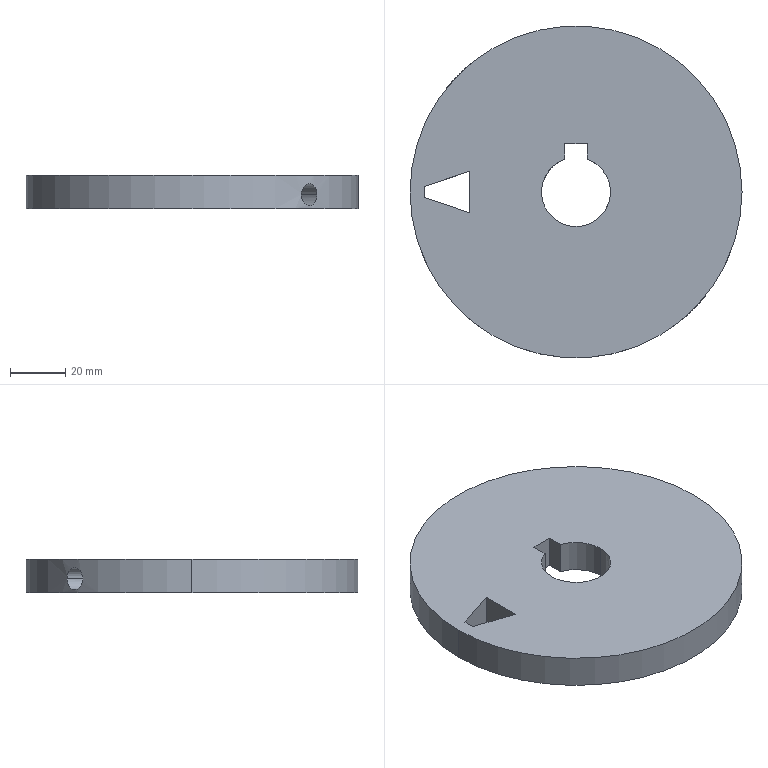Part | 1 solid | 24 faces | box 120 x 120 x 12 mm | volume 123752 mm3 | cylinder 13 | plane 11 | commonest cylinder face diameters 5 x4 8 x4 25 x3 120 x2
STEP:
#1=CARTESIAN_POINT('',(-45.16,39.504,5.));
#2=VERTEX_POINT('',#1);
#3=CARTESIAN_POINT('',(-39.504,45.16,5.));
#4=VERTEX_POINT('',#3);
#5=CARTESIAN_POINT('',(-45.16,39.504,5.));
#6=CARTESIAN_POINT('',(-45.16,39.504,4.739));
#7=CARTESIAN_POINT('',(-45.144,39.523,4.479));
#8=CARTESIAN_POINT('',(-45.076,39.6,3.964));
#9=CARTESIAN_POINT('',(-45.025,39.658,3.711));
#10=CARTESIAN_POINT('',(-44.893,39.807,3.23));
#11=CARTESIAN_POINT('',(-44.811,39.9,2.997));
#12=CARTESIAN_POINT('',(-44.616,40.118,2.559));
#13=CARTESIAN_POINT('',(-44.505,40.241,2.358));
#14=CARTESIAN_POINT('',(-44.256,40.514,1.989));
#15=CARTESIAN_POINT('',(-44.117,40.666,1.82));
#16=CARTESIAN_POINT('',(-43.821,40.985,1.529));
#17=CARTESIAN_POINT('',(-43.664,41.152,1.406));
#18=CARTESIAN_POINT('',(-43.331,41.503,1.206));
#19=CARTESIAN_POINT('',(-43.155,41.686,1.128));
#20=CARTESIAN_POINT('',(-42.798,42.053,1.026));
#21=CARTESIAN_POINT('',(-42.615,42.237,1.));
#22=CARTESIAN_POINT('',(-42.242,42.611,0.9998));
#23=CARTESIAN_POINT('',(-42.056,42.794,1.026));
#24=CARTESIAN_POINT('',(-41.69,43.151,1.127));
#25=CARTESIAN_POINT('',(-41.507,43.327,1.203));
#26=CARTESIAN_POINT('',(-41.156,43.661,1.404));
#27=CARTESIAN_POINT('',(-40.988,43.818,1.527));
#28=CARTESIAN_POINT('',(-40.669,44.114,1.816));
#29=CARTESIAN_POINT('',(-40.517,44.253,1.985));
#30=CARTESIAN_POINT('',(-40.244,44.502,2.354));
#31=CARTESIAN_POINT('',(-40.121,44.613,2.555));
#32=CARTESIAN_POINT('',(-39.902,44.809,2.992));
#33=CARTESIAN_POINT('',(-39.809,44.892,3.225));
#34=CARTESIAN_POINT('',(-39.659,45.024,3.706));
#35=CARTESIAN_POINT('',(-39.601,45.075,3.957));
#36=CARTESIAN_POINT('',(-39.523,45.143,4.474));
#37=CARTESIAN_POINT('',(-39.504,45.16,4.736));
#38=CARTESIAN_POINT('',(-39.504,45.16,5.));
#39=B_SPLINE_CURVE_WITH_KNOTS('',3,(#5,#6,#7,#8,#9,#10,#11,#12,#13,#14,#15,#16,#17,#18,#19,#20,#21,#22,#23,#24,#25,#26,#27,#28,#29,#30,#31,#32,#33,#34,#35,#36,#37,#38),.UNSPECIFIED.,.F.,.F.,(4,2,2,2,2,2,2,2,2,2,2,2,2,2,2,2,4),(0.01251,0.01329,0.01407,0.01485,0.01564,0.01642,0.0172,0.01798,0.01876,0.01954,0.02033,0.02111,0.02189,0.02267,0.02345,0.02423,0.02502),.UNSPECIFIED.);
#40=EDGE_CURVE('',#2,#4,#39,.T.);
#41=ORIENTED_EDGE('',*,*,#40,.F.);
#42=CARTESIAN_POINT('',(-24.042,18.385,5.));
#43=VERTEX_POINT('',#42);
#44=CARTESIAN_POINT('',(-58.69,53.033,5.));
#45=DIRECTION('',(0.7071,-0.7071,0.));
#46=VECTOR('',#45,1000.);
#47=LINE('',#44,#46);
#48=EDGE_CURVE('',#2,#43,#47,.T.);
#49=ORIENTED_EDGE('',*,*,#48,.T.);
#50=CARTESIAN_POINT('',(-18.385,24.042,5.));
#51=VERTEX_POINT('',#50);
#52=CARTESIAN_POINT('',(-21.213,21.213,5.));
#53=DIRECTION('',(0.7071,-0.7071,0.));
#54=DIRECTION('',(0.7071,0.7071,0.));
#55=AXIS2_PLACEMENT_3D('',#52,#53,#54);
#56=CIRCLE('',#55,4.);
#57=EDGE_CURVE('',#43,#51,#56,.T.);
#58=ORIENTED_EDGE('',*,*,#57,.T.);
#59=CARTESIAN_POINT('',(-53.033,58.69,5.));
#60=DIRECTION('',(0.7071,-0.7071,0.));
#61=VECTOR('',#60,1000.);
#62=LINE('',#59,#61);
#63=EDGE_CURVE('',#4,#51,#62,.T.);
#64=ORIENTED_EDGE('',*,*,#63,.F.);
#65=EDGE_LOOP('',(#41,#49,#58,#64));
#66=FACE_OUTER_BOUND('',#65,.T.);
#67=CARTESIAN_POINT('',(-55.861,55.861,5.));
#68=DIRECTION('',(0.7071,-0.7071,0.));
#69=DIRECTION('',(0.7071,0.7071,0.));
#70=AXIS2_PLACEMENT_3D('',#67,#68,#69);
#71=CYLINDRICAL_SURFACE('',#70,4.);
#72=ADVANCED_FACE('',(#66),#71,.F.);
#73=CARTESIAN_POINT('',(39.504,-45.16,5.));
#74=VERTEX_POINT('',#73);
#75=CARTESIAN_POINT('',(45.16,-39.504,5.));
#76=VERTEX_POINT('',#75);
#77=CARTESIAN_POINT('',(39.504,-45.16,5.));
#78=CARTESIAN_POINT('',(39.504,-45.16,4.736));
#79=CARTESIAN_POINT('',(39.523,-45.143,4.476));
#80=CARTESIAN_POINT('',(39.6,-45.076,3.964));
#81=CARTESIAN_POINT('',(39.658,-45.025,3.71));
#82=CARTESIAN_POINT('',(39.809,-44.892,3.226));
#83=CARTESIAN_POINT('',(39.901,-44.81,2.996));
#84=CARTESIAN_POINT('',(40.117,-44.616,2.561));
#85=CARTESIAN_POINT('',(40.243,-44.503,2.355));
#86=CARTESIAN_POINT('',(40.516,-44.255,1.987));
#87=CARTESIAN_POINT('',(40.665,-44.118,1.821));
#88=CARTESIAN_POINT('',(40.985,-43.821,1.529));
#89=CARTESIAN_POINT('',(41.155,-43.661,1.404));
#90=CARTESIAN_POINT('',(41.504,-43.33,1.205));
#91=CARTESIAN_POINT('',(41.686,-43.155,1.128));
#92=CARTESIAN_POINT('',(42.056,-42.794,1.025));
#93=CARTESIAN_POINT('',(42.241,-42.612,1.));
#94=CARTESIAN_POINT('',(42.61,-42.243,0.9999));
#95=CARTESIAN_POINT('',(42.796,-42.054,1.026));
#96=CARTESIAN_POINT('',(43.154,-41.687,1.128));
#97=CARTESIAN_POINT('',(43.327,-41.507,1.204));
#98=CARTESIAN_POINT('',(43.661,-41.156,1.404));
#99=CARTESIAN_POINT('',(43.821,-40.985,1.529));
#100=CARTESIAN_POINT('',(44.116,-40.667,1.819));
#101=CARTESIAN_POINT('',(44.253,-40.518,1.984));
#102=CARTESIAN_POINT('',(44.505,-40.241,2.358));
#103=CARTESIAN_POINT('',(44.616,-40.118,2.56));
#104=CARTESIAN_POINT('',(44.809,-39.902,2.993));
#105=CARTESIAN_POINT('',(44.892,-39.808,3.227));
#106=CARTESIAN_POINT('',(45.026,-39.657,3.712));
#107=CARTESIAN_POINT('',(45.076,-39.6,3.961));
#108=CARTESIAN_POINT('',(45.143,-39.523,4.474));
#109=CARTESIAN_POINT('',(45.16,-39.504,4.739));
#110=CARTESIAN_POINT('',(45.16,-39.504,5.));
#111=B_SPLINE_CURVE_WITH_KNOTS('',3,(#77,#78,#79,#80,#81,#82,#83,#84,#85,#86,#87,#88,#89,#90,#91,#92,#93,#94,#95,#96,#97,#98,#99,#100,#101,#102,#103,#104,#105,#106,#107,#108,#109,#110),.UNSPECIFIED.,.F.,.F.,(4,2,2,2,2,2,2,2,2,2,2,2,2,2,2,2,4),(0.,0.0007818,0.001564,0.002345,0.003127,0.003909,0.004691,0.005473,0.006255,0.007036,0.007818,0.0086,0.009382,0.01016,0.01095,0.01173,0.01251),.UNSPECIFIED.);
#112=EDGE_CURVE('',#74,#76,#111,.T.);
#113=ORIENTED_EDGE('',*,*,#112,.T.);
#114=CARTESIAN_POINT('',(24.042,-18.385,5.));
#115=VERTEX_POINT('',#114);
#116=CARTESIAN_POINT('',(58.69,-53.033,5.));
#117=DIRECTION('',(-0.7071,0.7071,0.));
#118=VECTOR('',#117,1000.);
#119=LINE('',#116,#118);
#120=EDGE_CURVE('',#76,#115,#119,.T.);
#121=ORIENTED_EDGE('',*,*,#120,.T.);
#122=CARTESIAN_POINT('',(18.385,-24.042,5.));
#123=VERTEX_POINT('',#122);
#124=CARTESIAN_POINT('',(21.213,-21.213,5.));
#125=DIRECTION('',(0.7071,-0.7071,0.));
#126=DIRECTION('',(0.7071,0.7071,0.));
#127=AXIS2_PLACEMENT_3D('',#124,#125,#126);
#128=CIRCLE('',#127,4.);
#129=EDGE_CURVE('',#123,#115,#128,.T.);
#130=ORIENTED_EDGE('',*,*,#129,.F.);
#131=CARTESIAN_POINT('',(53.033,-58.69,5.));
#132=DIRECTION('',(-0.7071,0.7071,0.));
#133=VECTOR('',#132,1000.);
#134=LINE('',#131,#133);
#135=EDGE_CURVE('',#74,#123,#134,.T.);
#136=ORIENTED_EDGE('',*,*,#135,.F.);
#137=EDGE_LOOP('',(#113,#121,#130,#136));
#138=FACE_OUTER_BOUND('',#137,.T.);
#139=CARTESIAN_POINT('',(55.861,-55.861,5.));
#140=DIRECTION('',(-0.7071,0.7071,0.));
#141=DIRECTION('',(-0.7071,-0.7071,0.));
#142=AXIS2_PLACEMENT_3D('',#139,#140,#141);
#143=CYLINDRICAL_SURFACE('',#142,4.);
#144=ADVANCED_FACE('',(#138),#143,.F.);
#145=CARTESIAN_POINT('',(6.892,-10.428,5.));
#146=VERTEX_POINT('',#145);
#147=CARTESIAN_POINT('',(10.428,-6.892,5.));
#148=VERTEX_POINT('',#147);
#149=CARTESIAN_POINT('',(6.892,-10.428,5.));
#150=CARTESIAN_POINT('',(6.892,-10.428,4.834));
#151=CARTESIAN_POINT('',(6.906,-10.419,4.672));
#152=CARTESIAN_POINT('',(6.961,-10.383,4.351));
#153=CARTESIAN_POINT('',(7.001,-10.355,4.192));
#154=CARTESIAN_POINT('',(7.107,-10.283,3.89));
#155=CARTESIAN_POINT('',(7.171,-10.239,3.746));
#156=CARTESIAN_POINT('',(7.321,-10.132,3.475));
#157=CARTESIAN_POINT('',(7.407,-10.069,3.347));
#158=CARTESIAN_POINT('',(7.686,-9.86,3.002));
#159=CARTESIAN_POINT('',(7.906,-9.687,2.816));
#160=CARTESIAN_POINT('',(8.25,-9.392,2.629));
#161=CARTESIAN_POINT('',(8.368,-9.287,2.58));
#162=CARTESIAN_POINT('',(8.605,-9.068,2.516));
#163=CARTESIAN_POINT('',(8.723,-8.955,2.5));
#164=CARTESIAN_POINT('',(8.954,-8.724,2.5));
#165=CARTESIAN_POINT('',(9.069,-8.604,2.516));
#166=CARTESIAN_POINT('',(9.287,-8.368,2.58));
#167=CARTESIAN_POINT('',(9.391,-8.251,2.628));
#168=CARTESIAN_POINT('',(9.589,-8.02,2.753));
#169=CARTESIAN_POINT('',(9.682,-7.908,2.832));
#170=CARTESIAN_POINT('',(9.852,-7.695,3.012));
#171=CARTESIAN_POINT('',(9.93,-7.594,3.116));
#172=CARTESIAN_POINT('',(10.071,-7.406,3.349));
#173=CARTESIAN_POINT('',(10.132,-7.321,3.474));
#174=CARTESIAN_POINT('',(10.238,-7.172,3.745));
#175=CARTESIAN_POINT('',(10.284,-7.106,3.891));
#176=CARTESIAN_POINT('',(10.356,-7.001,4.193));
#177=CARTESIAN_POINT('',(10.382,-6.961,4.349));
#178=CARTESIAN_POINT('',(10.419,-6.906,4.671));
#179=CARTESIAN_POINT('',(10.428,-6.892,4.837));
#180=CARTESIAN_POINT('',(10.428,-6.892,5.));
#181=B_SPLINE_CURVE_WITH_KNOTS('',3,(#149,#150,#151,#152,#153,#154,#155,#156,#157,#158,#159,#160,#161,#162,#163,#164,#165,#166,#167,#168,#169,#170,#171,#172,#173,#174,#175,#176,#177,#178,#179,#180),.UNSPECIFIED.,.F.,.F.,(4,2,2,2,2,2,2,2,2,2,2,2,2,2,2,4),(0.,0.0004897,0.0009795,0.001469,0.001959,0.002938,0.003428,0.003918,0.004408,0.004897,0.005387,0.005877,0.006367,0.006856,0.007346,0.007836),.UNSPECIFIED.);
#182=EDGE_CURVE('',#146,#148,#181,.T.);
#183=ORIENTED_EDGE('',*,*,#182,.T.);
#184=CARTESIAN_POINT('',(10.428,-6.892,5.));
#185=CARTESIAN_POINT('',(10.428,-6.892,5.327));
#186=CARTESIAN_POINT('',(10.391,-6.949,5.656));
#187=CARTESIAN_POINT('',(10.284,-7.106,6.108));
#188=CARTESIAN_POINT('',(10.239,-7.171,6.254));
#189=CARTESIAN_POINT('',(10.132,-7.322,6.526));
#190=CARTESIAN_POINT('',(10.07,-7.406,6.651));
#191=CARTESIAN_POINT('',(9.931,-7.592,6.882));
#192=CARTESIAN_POINT('',(9.852,-7.695,6.987));
#193=CARTESIAN_POINT('',(9.682,-7.907,7.168));
#194=CARTESIAN_POINT('',(9.59,-8.019,7.245));
#195=CARTESIAN_POINT('',(9.293,-8.365,7.435));
#196=CARTESIAN_POINT('',(9.073,-8.605,7.5));
#197=CARTESIAN_POINT('',(8.723,-8.955,7.5));
#198=CARTESIAN_POINT('',(8.606,-9.067,7.484));
#199=CARTESIAN_POINT('',(8.37,-9.285,7.42));
#200=CARTESIAN_POINT('',(8.251,-9.391,7.372));
#201=CARTESIAN_POINT('',(8.021,-9.588,7.247));
#202=CARTESIAN_POINT('',(7.91,-9.68,7.17));
#203=CARTESIAN_POINT('',(7.696,-9.851,6.989));
#204=CARTESIAN_POINT('',(7.594,-9.93,6.884));
#205=CARTESIAN_POINT('',(7.315,-10.139,6.539));
#206=CARTESIAN_POINT('',(7.16,-10.247,6.261));
#207=CARTESIAN_POINT('',(7.002,-10.355,5.81));
#208=CARTESIAN_POINT('',(6.961,-10.382,5.652));
#209=CARTESIAN_POINT('',(6.906,-10.419,5.329));
#210=CARTESIAN_POINT('',(6.892,-10.428,5.166));
#211=CARTESIAN_POINT('',(6.892,-10.428,5.));
#212=B_SPLINE_CURVE_WITH_KNOTS('',3,(#184,#185,#186,#187,#188,#189,#190,#191,#192,#193,#194,#195,#196,#197,#198,#199,#200,#201,#202,#203,#204,#205,#206,#207,#208,#209,#210,#211),.UNSPECIFIED.,.F.,.F.,(4,2,2,2,2,2,2,2,2,2,2,2,2,4),(0.007836,0.008815,0.009305,0.009794,0.01028,0.01077,0.01175,0.01224,0.01273,0.01322,0.01371,0.01469,0.01518,0.01567),.UNSPECIFIED.);
#213=EDGE_CURVE('',#148,#146,#212,.T.);
#214=ORIENTED_EDGE('',*,*,#213,.T.);
#215=EDGE_LOOP('',(#183,#214));
#216=FACE_BOUND('',#215,.T.);
#217=CARTESIAN_POINT('',(-12.5,0.,12.));
#218=VERTEX_POINT('',#217);
#219=CARTESIAN_POINT('',(12.5,0.,12.));
#220=VERTEX_POINT('',#219);
#221=CARTESIAN_POINT('',(0.,0.,12.));
#222=DIRECTION('',(0.,0.,1.));
#223=DIRECTION('',(1.,0.,0.));
#224=AXIS2_PLACEMENT_3D('',#221,#222,#223);
#225=CIRCLE('',#224,12.5);
#226=EDGE_CURVE('',#218,#220,#225,.T.);
#227=ORIENTED_EDGE('',*,*,#226,.T.);
#228=CARTESIAN_POINT('',(12.5,0.,0.));
#229=VERTEX_POINT('',#228);
#230=CARTESIAN_POINT('',(12.5,0.,12.));
#231=DIRECTION('',(0.,0.,-1.));
#232=VECTOR('',#231,1000.);
#233=LINE('',#230,#232);
#234=EDGE_CURVE('',#220,#229,#233,.T.);
#235=ORIENTED_EDGE('',*,*,#234,.T.);
#236=CARTESIAN_POINT('',(-12.5,0.,0.));
#237=VERTEX_POINT('',#236);
#238=CARTESIAN_POINT('',(0.,0.,0.));
#239=DIRECTION('',(0.,0.,1.));
#240=DIRECTION('',(1.,0.,0.));
#241=AXIS2_PLACEMENT_3D('',#238,#239,#240);
#242=CIRCLE('',#241,12.5);
#243=EDGE_CURVE('',#237,#229,#242,.T.);
#244=ORIENTED_EDGE('',*,*,#243,.F.);
#245=CARTESIAN_POINT('',(-12.5,0.,12.));
#246=DIRECTION('',(0.,0.,-1.));
#247=VECTOR('',#246,1000.);
#248=LINE('',#245,#247);
#249=EDGE_CURVE('',#218,#237,#248,.T.);
#250=ORIENTED_EDGE('',*,*,#249,.F.);
#251=EDGE_LOOP('',(#227,#235,#244,#250));
#252=FACE_OUTER_BOUND('',#251,.T.);
#253=CARTESIAN_POINT('',(0.,0.,12.));
#254=DIRECTION('',(0.,0.,-1.));
#255=DIRECTION('',(-1.,0.,0.));
#256=AXIS2_PLACEMENT_3D('',#253,#254,#255);
#257=CYLINDRICAL_SURFACE('',#256,12.5);
#258=ADVANCED_FACE('',(#216,#252),#257,.F.);
#259=CARTESIAN_POINT('',(-10.428,6.892,5.));
#260=VERTEX_POINT('',#259);
#261=CARTESIAN_POINT('',(-6.892,10.428,5.));
#262=VERTEX_POINT('',#261);
#263=CARTESIAN_POINT('',(-10.428,6.892,5.));
#264=CARTESIAN_POINT('',(-10.428,6.892,5.166));
#265=CARTESIAN_POINT('',(-10.419,6.906,5.328));
#266=CARTESIAN_POINT('',(-10.383,6.961,5.649));
#267=CARTESIAN_POINT('',(-10.355,7.001,5.808));
#268=CARTESIAN_POINT('',(-10.283,7.107,6.11));
#269=CARTESIAN_POINT('',(-10.239,7.171,6.254));
#270=CARTESIAN_POINT('',(-10.132,7.321,6.525));
#271=CARTESIAN_POINT('',(-10.069,7.407,6.653));
#272=CARTESIAN_POINT('',(-9.86,7.686,6.998));
#273=CARTESIAN_POINT('',(-9.687,7.906,7.184));
#274=CARTESIAN_POINT('',(-9.392,8.25,7.371));
#275=CARTESIAN_POINT('',(-9.287,8.368,7.42));
#276=CARTESIAN_POINT('',(-9.068,8.605,7.484));
#277=CARTESIAN_POINT('',(-8.955,8.723,7.5));
#278=CARTESIAN_POINT('',(-8.724,8.954,7.5));
#279=CARTESIAN_POINT('',(-8.604,9.069,7.484));
#280=CARTESIAN_POINT('',(-8.368,9.287,7.42));
#281=CARTESIAN_POINT('',(-8.251,9.391,7.372));
#282=CARTESIAN_POINT('',(-8.02,9.589,7.247));
#283=CARTESIAN_POINT('',(-7.908,9.682,7.168));
#284=CARTESIAN_POINT('',(-7.695,9.852,6.988));
#285=CARTESIAN_POINT('',(-7.594,9.93,6.884));
#286=CARTESIAN_POINT('',(-7.406,10.071,6.651));
#287=CARTESIAN_POINT('',(-7.321,10.132,6.526));
#288=CARTESIAN_POINT('',(-7.172,10.238,6.255));
#289=CARTESIAN_POINT('',(-7.106,10.284,6.109));
#290=CARTESIAN_POINT('',(-7.001,10.356,5.807));
#291=CARTESIAN_POINT('',(-6.961,10.382,5.651));
#292=CARTESIAN_POINT('',(-6.906,10.419,5.329));
#293=CARTESIAN_POINT('',(-6.892,10.428,5.163));
#294=CARTESIAN_POINT('',(-6.892,10.428,5.));
#295=B_SPLINE_CURVE_WITH_KNOTS('',3,(#263,#264,#265,#266,#267,#268,#269,#270,#271,#272,#273,#274,#275,#276,#277,#278,#279,#280,#281,#282,#283,#284,#285,#286,#287,#288,#289,#290,#291,#292,#293,#294),.UNSPECIFIED.,.F.,.F.,(4,2,2,2,2,2,2,2,2,2,2,2,2,2,2,4),(0.,0.0004897,0.0009795,0.001469,0.001959,0.002938,0.003428,0.003918,0.004408,0.004897,0.005387,0.005877,0.006367,0.006856,0.007346,0.007836),.UNSPECIFIED.);
#296=EDGE_CURVE('',#260,#262,#295,.T.);
#297=ORIENTED_EDGE('',*,*,#296,.T.);
#298=CARTESIAN_POINT('',(-6.892,10.428,5.));
#299=CARTESIAN_POINT('',(-6.892,10.428,4.673));
#300=CARTESIAN_POINT('',(-6.949,10.391,4.344));
#301=CARTESIAN_POINT('',(-7.106,10.284,3.892));
#302=CARTESIAN_POINT('',(-7.171,10.239,3.746));
#303=CARTESIAN_POINT('',(-7.322,10.132,3.474));
#304=CARTESIAN_POINT('',(-7.406,10.07,3.349));
#305=CARTESIAN_POINT('',(-7.592,9.931,3.118));
#306=CARTESIAN_POINT('',(-7.695,9.852,3.013));
#307=CARTESIAN_POINT('',(-7.907,9.682,2.832));
#308=CARTESIAN_POINT('',(-8.019,9.59,2.755));
#309=CARTESIAN_POINT('',(-8.365,9.293,2.565));
#310=CARTESIAN_POINT('',(-8.605,9.073,2.5));
#311=CARTESIAN_POINT('',(-8.955,8.723,2.5));
#312=CARTESIAN_POINT('',(-9.067,8.606,2.516));
#313=CARTESIAN_POINT('',(-9.285,8.37,2.58));
#314=CARTESIAN_POINT('',(-9.391,8.251,2.628));
#315=CARTESIAN_POINT('',(-9.588,8.021,2.753));
#316=CARTESIAN_POINT('',(-9.68,7.91,2.83));
#317=CARTESIAN_POINT('',(-9.851,7.696,3.011));
#318=CARTESIAN_POINT('',(-9.93,7.594,3.116));
#319=CARTESIAN_POINT('',(-10.139,7.315,3.461));
#320=CARTESIAN_POINT('',(-10.247,7.16,3.739));
#321=CARTESIAN_POINT('',(-10.355,7.002,4.19));
#322=CARTESIAN_POINT('',(-10.382,6.961,4.348));
#323=CARTESIAN_POINT('',(-10.419,6.906,4.671));
#324=CARTESIAN_POINT('',(-10.428,6.892,4.834));
#325=CARTESIAN_POINT('',(-10.428,6.892,5.));
#326=B_SPLINE_CURVE_WITH_KNOTS('',3,(#298,#299,#300,#301,#302,#303,#304,#305,#306,#307,#308,#309,#310,#311,#312,#313,#314,#315,#316,#317,#318,#319,#320,#321,#322,#323,#324,#325),.UNSPECIFIED.,.F.,.F.,(4,2,2,2,2,2,2,2,2,2,2,2,2,4),(0.007836,0.008815,0.009305,0.009794,0.01028,0.01077,0.01175,0.01224,0.01273,0.01322,0.01371,0.01469,0.01518,0.01567),.UNSPECIFIED.);
#327=EDGE_CURVE('',#262,#260,#326,.T.);
#328=ORIENTED_EDGE('',*,*,#327,.T.);
#329=EDGE_LOOP('',(#297,#328));
#330=FACE_BOUND('',#329,.T.);
#331=CARTESIAN_POINT('',(-4.,11.843,12.));
#332=VERTEX_POINT('',#331);
#333=CARTESIAN_POINT('',(0.,0.,12.));
#334=DIRECTION('',(0.,0.,1.));
#335=DIRECTION('',(1.,0.,0.));
#336=AXIS2_PLACEMENT_3D('',#333,#334,#335);
#337=CIRCLE('',#336,12.5);
#338=EDGE_CURVE('',#332,#218,#337,.T.);
#339=ORIENTED_EDGE('',*,*,#338,.T.);
#340=ORIENTED_EDGE('',*,*,#249,.T.);
#341=CARTESIAN_POINT('',(-4.,11.843,0.));
#342=VERTEX_POINT('',#341);
#343=CARTESIAN_POINT('',(0.,0.,0.));
#344=DIRECTION('',(0.,0.,1.));
#345=DIRECTION('',(1.,0.,0.));
#346=AXIS2_PLACEMENT_3D('',#343,#344,#345);
#347=CIRCLE('',#346,12.5);
#348=EDGE_CURVE('',#342,#237,#347,.T.);
#349=ORIENTED_EDGE('',*,*,#348,.F.);
#350=CARTESIAN_POINT('',(-4.,11.843,12.));
#351=DIRECTION('',(0.,0.,-1.));
#352=VECTOR('',#351,1000.);
#353=LINE('',#350,#352);
#354=EDGE_CURVE('',#332,#342,#353,.T.);
#355=ORIENTED_EDGE('',*,*,#354,.F.);
#356=EDGE_LOOP('',(#339,#340,#349,#355));
#357=FACE_OUTER_BOUND('',#356,.T.);
#358=CARTESIAN_POINT('',(0.,0.,12.));
#359=DIRECTION('',(0.,0.,-1.));
#360=DIRECTION('',(-1.,0.,0.));
#361=AXIS2_PLACEMENT_3D('',#358,#359,#360);
#362=CYLINDRICAL_SURFACE('',#361,12.5);
#363=ADVANCED_FACE('',(#330,#357),#362,.F.);
#364=CARTESIAN_POINT('',(19.445,-22.981,5.));
#365=VERTEX_POINT('',#364);
#366=CARTESIAN_POINT('',(22.981,-19.445,5.));
#367=VERTEX_POINT('',#366);
#368=CARTESIAN_POINT('',(21.213,-21.213,5.));
#369=DIRECTION('',(0.7071,-0.7071,0.));
#370=DIRECTION('',(0.7071,0.7071,0.));
#371=AXIS2_PLACEMENT_3D('',#368,#369,#370);
#372=CIRCLE('',#371,2.5);
#373=EDGE_CURVE('',#365,#367,#372,.T.);
#374=ORIENTED_EDGE('',*,*,#373,.T.);
#375=CARTESIAN_POINT('',(129.047,-125.511,5.));
#376=DIRECTION('',(-0.7071,0.7071,0.));
#377=VECTOR('',#376,1000.);
#378=LINE('',#375,#377);
#379=EDGE_CURVE('',#367,#148,#378,.T.);
#380=ORIENTED_EDGE('',*,*,#379,.T.);
#381=ORIENTED_EDGE('',*,*,#182,.F.);
#382=CARTESIAN_POINT('',(125.511,-129.047,5.));
#383=DIRECTION('',(-0.7071,0.7071,0.));
#384=VECTOR('',#383,1000.);
#385=LINE('',#382,#384);
#386=EDGE_CURVE('',#365,#146,#385,.T.);
#387=ORIENTED_EDGE('',*,*,#386,.F.);
#388=EDGE_LOOP('',(#374,#380,#381,#387));
#389=FACE_OUTER_BOUND('',#388,.T.);
#390=CARTESIAN_POINT('',(127.279,-127.279,5.));
#391=DIRECTION('',(-0.7071,0.7071,0.));
#392=DIRECTION('',(-0.7071,-0.7071,0.));
#393=AXIS2_PLACEMENT_3D('',#390,#391,#392);
#394=CYLINDRICAL_SURFACE('',#393,2.5);
#395=ADVANCED_FACE('',(#389),#394,.F.);
#396=CARTESIAN_POINT('',(-39.504,45.16,5.));
#397=CARTESIAN_POINT('',(-39.504,45.16,5.264));
#398=CARTESIAN_POINT('',(-39.523,45.143,5.524));
#399=CARTESIAN_POINT('',(-39.6,45.076,6.036));
#400=CARTESIAN_POINT('',(-39.658,45.025,6.29));
#401=CARTESIAN_POINT('',(-39.809,44.892,6.774));
#402=CARTESIAN_POINT('',(-39.901,44.81,7.004));
#403=CARTESIAN_POINT('',(-40.117,44.616,7.439));
#404=CARTESIAN_POINT('',(-40.243,44.503,7.645));
#405=CARTESIAN_POINT('',(-40.516,44.255,8.013));
#406=CARTESIAN_POINT('',(-40.665,44.118,8.179));
#407=CARTESIAN_POINT('',(-40.985,43.821,8.471));
#408=CARTESIAN_POINT('',(-41.155,43.661,8.596));
#409=CARTESIAN_POINT('',(-41.504,43.33,8.795));
#410=CARTESIAN_POINT('',(-41.686,43.155,8.872));
#411=CARTESIAN_POINT('',(-42.056,42.794,8.975));
#412=CARTESIAN_POINT('',(-42.241,42.612,9.));
#413=CARTESIAN_POINT('',(-42.61,42.243,9.));
#414=CARTESIAN_POINT('',(-42.796,42.054,8.974));
#415=CARTESIAN_POINT('',(-43.154,41.687,8.872));
#416=CARTESIAN_POINT('',(-43.327,41.507,8.796));
#417=CARTESIAN_POINT('',(-43.661,41.156,8.596));
#418=CARTESIAN_POINT('',(-43.821,40.985,8.471));
#419=CARTESIAN_POINT('',(-44.116,40.667,8.181));
#420=CARTESIAN_POINT('',(-44.253,40.518,8.016));
#421=CARTESIAN_POINT('',(-44.505,40.241,7.642));
#422=CARTESIAN_POINT('',(-44.616,40.118,7.44));
#423=CARTESIAN_POINT('',(-44.809,39.902,7.007));
#424=CARTESIAN_POINT('',(-44.892,39.808,6.773));
#425=CARTESIAN_POINT('',(-45.026,39.657,6.288));
#426=CARTESIAN_POINT('',(-45.076,39.6,6.039));
#427=CARTESIAN_POINT('',(-45.143,39.523,5.526));
#428=CARTESIAN_POINT('',(-45.16,39.504,5.261));
#429=CARTESIAN_POINT('',(-45.16,39.504,5.));
#430=B_SPLINE_CURVE_WITH_KNOTS('',3,(#396,#397,#398,#399,#400,#401,#402,#403,#404,#405,#406,#407,#408,#409,#410,#411,#412,#413,#414,#415,#416,#417,#418,#419,#420,#421,#422,#423,#424,#425,#426,#427,#428,#429),.UNSPECIFIED.,.F.,.F.,(4,2,2,2,2,2,2,2,2,2,2,2,2,2,2,2,4),(0.,0.0007818,0.001564,0.002345,0.003127,0.003909,0.004691,0.005473,0.006255,0.007036,0.007818,0.0086,0.009382,0.01016,0.01095,0.01173,0.01251),.UNSPECIFIED.);
#431=EDGE_CURVE('',#4,#2,#430,.T.);
#432=ORIENTED_EDGE('',*,*,#431,.T.);
#433=ORIENTED_EDGE('',*,*,#40,.T.);
#434=EDGE_LOOP('',(#432,#433));
#435=FACE_BOUND('',#434,.T.);
#436=CARTESIAN_POINT('',(60.,0.,12.));
#437=VERTEX_POINT('',#436);
#438=CARTESIAN_POINT('',(-60.,0.,12.));
#439=VERTEX_POINT('',#438);
#440=CARTESIAN_POINT('',(0.,0.,12.));
#441=DIRECTION('',(0.,0.,1.));
#442=DIRECTION('',(1.,0.,0.));
#443=AXIS2_PLACEMENT_3D('',#440,#441,#442);
#444=CIRCLE('',#443,60.);
#445=EDGE_CURVE('',#437,#439,#444,.T.);
#446=ORIENTED_EDGE('',*,*,#445,.F.);
#447=CARTESIAN_POINT('',(60.,0.,0.));
#448=VERTEX_POINT('',#447);
#449=CARTESIAN_POINT('',(60.,0.,12.));
#450=DIRECTION('',(0.,0.,-1.));
#451=VECTOR('',#450,1000.);
#452=LINE('',#449,#451);
#453=EDGE_CURVE('',#437,#448,#452,.T.);
#454=ORIENTED_EDGE('',*,*,#453,.T.);
#455=CARTESIAN_POINT('',(-60.,0.,0.));
#456=VERTEX_POINT('',#455);
#457=CARTESIAN_POINT('',(0.,0.,0.));
#458=DIRECTION('',(0.,0.,1.));
#459=DIRECTION('',(1.,0.,0.));
#460=AXIS2_PLACEMENT_3D('',#457,#458,#459);
#461=CIRCLE('',#460,60.);
#462=EDGE_CURVE('',#448,#456,#461,.T.);
#463=ORIENTED_EDGE('',*,*,#462,.T.);
#464=CARTESIAN_POINT('',(-60.,0.,12.));
#465=DIRECTION('',(0.,0.,-1.));
#466=VECTOR('',#465,1000.);
#467=LINE('',#464,#466);
#468=EDGE_CURVE('',#439,#456,#467,.T.);
#469=ORIENTED_EDGE('',*,*,#468,.F.);
#470=EDGE_LOOP('',(#446,#454,#463,#469));
#471=FACE_OUTER_BOUND('',#470,.T.);
#472=CARTESIAN_POINT('',(0.,0.,12.));
#473=DIRECTION('',(0.,0.,-1.));
#474=DIRECTION('',(-1.,0.,0.));
#475=AXIS2_PLACEMENT_3D('',#472,#473,#474);
#476=CYLINDRICAL_SURFACE('',#475,60.);
#477=ADVANCED_FACE('',(#435,#471),#476,.T.);
#478=ORIENTED_EDGE('',*,*,#327,.F.);
#479=CARTESIAN_POINT('',(-19.445,22.981,5.));
#480=VERTEX_POINT('',#479);
#481=CARTESIAN_POINT('',(129.047,-125.511,5.));
#482=DIRECTION('',(-0.7071,0.7071,0.));
#483=VECTOR('',#482,1000.);
#484=LINE('',#481,#483);
#485=EDGE_CURVE('',#262,#480,#484,.T.);
#486=ORIENTED_EDGE('',*,*,#485,.T.);
#487=CARTESIAN_POINT('',(-22.981,19.445,5.));
#488=VERTEX_POINT('',#487);
#489=CARTESIAN_POINT('',(-21.213,21.213,5.));
#490=DIRECTION('',(-0.7071,0.7071,0.));
#491=DIRECTION('',(-0.7071,-0.7071,0.));
#492=AXIS2_PLACEMENT_3D('',#489,#490,#491);
#493=CIRCLE('',#492,2.5);
#494=EDGE_CURVE('',#480,#488,#493,.T.);
#495=ORIENTED_EDGE('',*,*,#494,.T.);
#496=CARTESIAN_POINT('',(125.511,-129.047,5.));
#497=DIRECTION('',(-0.7071,0.7071,0.));
#498=VECTOR('',#497,1000.);
#499=LINE('',#496,#498);
#500=EDGE_CURVE('',#260,#488,#499,.T.);
#501=ORIENTED_EDGE('',*,*,#500,.F.);
#502=EDGE_LOOP('',(#478,#486,#495,#501));
#503=FACE_OUTER_BOUND('',#502,.T.);
#504=CARTESIAN_POINT('',(127.279,-127.279,5.));
#505=DIRECTION('',(-0.7071,0.7071,0.));
#506=DIRECTION('',(-0.7071,-0.7071,0.));
#507=AXIS2_PLACEMENT_3D('',#504,#505,#506);
#508=CYLINDRICAL_SURFACE('',#507,2.5);
#509=ADVANCED_FACE('',(#503),#508,.F.);
#510=CARTESIAN_POINT('',(4.,17.5,12.));
#511=VERTEX_POINT('',#510);
#512=CARTESIAN_POINT('',(-4.,17.5,12.));
#513=VERTEX_POINT('',#512);
#514=CARTESIAN_POINT('',(-4.,17.5,12.));
#515=DIRECTION('',(-1.,0.,0.));
#516=VECTOR('',#515,1000.);
#517=LINE('',#514,#516);
#518=EDGE_CURVE('',#511,#513,#517,.T.);
#519=ORIENTED_EDGE('',*,*,#518,.F.);
#520=CARTESIAN_POINT('',(4.,11.843,12.));
#521=VERTEX_POINT('',#520);
#522=CARTESIAN_POINT('',(4.,11.843,12.));
#523=DIRECTION('',(0.,1.,0.));
#524=VECTOR('',#523,1000.);
#525=LINE('',#522,#524);
#526=EDGE_CURVE('',#521,#511,#525,.T.);
#527=ORIENTED_EDGE('',*,*,#526,.F.);
#528=CARTESIAN_POINT('',(0.,0.,12.));
#529=DIRECTION('',(0.,0.,1.));
#530=DIRECTION('',(1.,0.,0.));
#531=AXIS2_PLACEMENT_3D('',#528,#529,#530);
#532=CIRCLE('',#531,12.5);
#533=EDGE_CURVE('',#220,#521,#532,.T.);
#534=ORIENTED_EDGE('',*,*,#533,.F.);
#535=ORIENTED_EDGE('',*,*,#226,.F.);
#536=ORIENTED_EDGE('',*,*,#338,.F.);
#537=CARTESIAN_POINT('',(-4.,11.843,12.));
#538=DIRECTION('',(0.,-1.,0.));
#539=VECTOR('',#538,1000.);
#540=LINE('',#537,#539);
#541=EDGE_CURVE('',#513,#332,#540,.T.);
#542=ORIENTED_EDGE('',*,*,#541,.F.);
#543=EDGE_LOOP('',(#519,#527,#534,#535,#536,#542));
#544=FACE_BOUND('',#543,.T.);
#545=CARTESIAN_POINT('',(0.,0.,12.));
#546=DIRECTION('',(0.,0.,1.));
#547=DIRECTION('',(1.,0.,0.));
#548=AXIS2_PLACEMENT_3D('',#545,#546,#547);
#549=CIRCLE('',#548,60.);
#550=EDGE_CURVE('',#439,#437,#549,.T.);
#551=ORIENTED_EDGE('',*,*,#550,.T.);
#552=ORIENTED_EDGE('',*,*,#445,.T.);
#553=EDGE_LOOP('',(#551,#552));
#554=FACE_OUTER_BOUND('',#553,.T.);
#555=CARTESIAN_POINT('',(-38.386,-7.5,12.));
#556=VERTEX_POINT('',#555);
#557=CARTESIAN_POINT('',(-54.798,-2.,12.));
#558=VERTEX_POINT('',#557);
#559=CARTESIAN_POINT('',(-6.135,-18.308,12.));
#560=DIRECTION('',(-0.9482,0.3177,0.));
#561=VECTOR('',#560,1000.);
#562=LINE('',#559,#561);
#563=EDGE_CURVE('',#556,#558,#562,.T.);
#564=ORIENTED_EDGE('',*,*,#563,.T.);
#565=CARTESIAN_POINT('',(-54.798,2.,12.));
#566=VERTEX_POINT('',#565);
#567=CARTESIAN_POINT('',(-54.798,0.,12.));
#568=DIRECTION('',(0.,1.,0.));
#569=VECTOR('',#568,1000.);
#570=LINE('',#567,#569);
#571=EDGE_CURVE('',#558,#566,#570,.T.);
#572=ORIENTED_EDGE('',*,*,#571,.T.);
#573=CARTESIAN_POINT('',(-38.386,7.5,12.));
#574=VERTEX_POINT('',#573);
#575=CARTESIAN_POINT('',(-6.135,18.308,12.));
#576=DIRECTION('',(0.9482,0.3177,0.));
#577=VECTOR('',#576,1000.);
#578=LINE('',#575,#577);
#579=EDGE_CURVE('',#566,#574,#578,.T.);
#580=ORIENTED_EDGE('',*,*,#579,.T.);
#581=CARTESIAN_POINT('',(-38.386,0.,12.));
#582=DIRECTION('',(0.,-1.,0.));
#583=VECTOR('',#582,1000.);
#584=LINE('',#581,#583);
#585=EDGE_CURVE('',#574,#556,#584,.T.);
#586=ORIENTED_EDGE('',*,*,#585,.T.);
#587=EDGE_LOOP('',(#564,#572,#580,#586));
#588=FACE_BOUND('',#587,.T.);
#589=CARTESIAN_POINT('',(0.,0.,12.));
#590=DIRECTION('',(0.,0.,1.));
#591=DIRECTION('',(1.,0.,0.));
#592=AXIS2_PLACEMENT_3D('',#589,#590,#591);
#593=PLANE('',#592);
#594=ADVANCED_FACE('',(#544,#554,#588),#593,.T.);
#595=CARTESIAN_POINT('',(4.,11.843,0.));
#596=VERTEX_POINT('',#595);
#597=CARTESIAN_POINT('',(4.,17.5,0.));
#598=VERTEX_POINT('',#597);
#599=CARTESIAN_POINT('',(4.,11.843,0.));
#600=DIRECTION('',(0.,1.,0.));
#601=VECTOR('',#600,1000.);
#602=LINE('',#599,#601);
#603=EDGE_CURVE('',#596,#598,#602,.T.);
#604=ORIENTED_EDGE('',*,*,#603,.T.);
#605=CARTESIAN_POINT('',(-4.,17.5,0.));
#606=VERTEX_POINT('',#605);
#607=CARTESIAN_POINT('',(-4.,17.5,0.));
#608=DIRECTION('',(-1.,0.,0.));
#609=VECTOR('',#608,1000.);
#610=LINE('',#607,#609);
#611=EDGE_CURVE('',#598,#606,#610,.T.);
#612=ORIENTED_EDGE('',*,*,#611,.T.);
#613=CARTESIAN_POINT('',(-4.,11.843,0.));
#614=DIRECTION('',(0.,-1.,0.));
#615=VECTOR('',#614,1000.);
#616=LINE('',#613,#615);
#617=EDGE_CURVE('',#606,#342,#616,.T.);
#618=ORIENTED_EDGE('',*,*,#617,.T.);
#619=ORIENTED_EDGE('',*,*,#348,.T.);
#620=ORIENTED_EDGE('',*,*,#243,.T.);
#621=CARTESIAN_POINT('',(0.,0.,0.));
#622=DIRECTION('',(0.,0.,1.));
#623=DIRECTION('',(1.,0.,0.));
#624=AXIS2_PLACEMENT_3D('',#621,#622,#623);
#625=CIRCLE('',#624,12.5);
#626=EDGE_CURVE('',#229,#596,#625,.T.);
#627=ORIENTED_EDGE('',*,*,#626,.T.);
#628=EDGE_LOOP('',(#604,#612,#618,#619,#620,#627));
#629=FACE_BOUND('',#628,.T.);
#630=CARTESIAN_POINT('',(0.,0.,0.));
#631=DIRECTION('',(0.,0.,1.));
#632=DIRECTION('',(1.,0.,0.));
#633=AXIS2_PLACEMENT_3D('',#630,#631,#632);
#634=CIRCLE('',#633,60.);
#635=EDGE_CURVE('',#456,#448,#634,.T.);
#636=ORIENTED_EDGE('',*,*,#635,.F.);
#637=ORIENTED_EDGE('',*,*,#462,.F.);
#638=EDGE_LOOP('',(#636,#637));
#639=FACE_OUTER_BOUND('',#638,.T.);
#640=CARTESIAN_POINT('',(-54.798,2.,0.));
#641=VERTEX_POINT('',#640);
#642=CARTESIAN_POINT('',(-54.798,-2.,0.));
#643=VERTEX_POINT('',#642);
#644=CARTESIAN_POINT('',(-54.798,2.,0.));
#645=DIRECTION('',(0.,-1.,0.));
#646=VECTOR('',#645,1000.);
#647=LINE('',#644,#646);
#648=EDGE_CURVE('',#641,#643,#647,.T.);
#649=ORIENTED_EDGE('',*,*,#648,.T.);
#650=CARTESIAN_POINT('',(-38.386,-7.5,0.));
#651=VERTEX_POINT('',#650);
#652=CARTESIAN_POINT('',(-38.386,-7.5,0.));
#653=DIRECTION('',(0.9482,-0.3177,0.));
#654=VECTOR('',#653,1000.);
#655=LINE('',#652,#654);
#656=EDGE_CURVE('',#643,#651,#655,.T.);
#657=ORIENTED_EDGE('',*,*,#656,.T.);
#658=CARTESIAN_POINT('',(-38.386,7.5,0.));
#659=VERTEX_POINT('',#658);
#660=CARTESIAN_POINT('',(-38.386,7.5,0.));
#661=DIRECTION('',(0.,1.,0.));
#662=VECTOR('',#661,1000.);
#663=LINE('',#660,#662);
#664=EDGE_CURVE('',#651,#659,#663,.T.);
#665=ORIENTED_EDGE('',*,*,#664,.T.);
#666=CARTESIAN_POINT('',(-38.386,7.5,0.));
#667=DIRECTION('',(-0.9482,-0.3177,0.));
#668=VECTOR('',#667,1000.);
#669=LINE('',#666,#668);
#670=EDGE_CURVE('',#659,#641,#669,.T.);
#671=ORIENTED_EDGE('',*,*,#670,.T.);
#672=EDGE_LOOP('',(#649,#657,#665,#671));
#673=FACE_BOUND('',#672,.T.);
#674=CARTESIAN_POINT('',(0.,0.,0.));
#675=DIRECTION('',(0.,0.,1.));
#676=DIRECTION('',(1.,0.,0.));
#677=AXIS2_PLACEMENT_3D('',#674,#675,#676);
#678=PLANE('',#677);
#679=ADVANCED_FACE('',(#629,#639,#673),#678,.F.);
#680=ORIENTED_EDGE('',*,*,#485,.F.);
#681=ORIENTED_EDGE('',*,*,#296,.F.);
#682=ORIENTED_EDGE('',*,*,#500,.T.);
#683=CARTESIAN_POINT('',(-21.213,21.213,5.));
#684=DIRECTION('',(-0.7071,0.7071,0.));
#685=DIRECTION('',(-0.7071,-0.7071,0.));
#686=AXIS2_PLACEMENT_3D('',#683,#684,#685);
#687=CIRCLE('',#686,2.5);
#688=EDGE_CURVE('',#488,#480,#687,.T.);
#689=ORIENTED_EDGE('',*,*,#688,.T.);
#690=EDGE_LOOP('',(#680,#681,#682,#689));
#691=FACE_OUTER_BOUND('',#690,.T.);
#692=CARTESIAN_POINT('',(127.279,-127.279,5.));
#693=DIRECTION('',(-0.7071,0.7071,0.));
#694=DIRECTION('',(-0.7071,-0.7071,0.));
#695=AXIS2_PLACEMENT_3D('',#692,#693,#694);
#696=CYLINDRICAL_SURFACE('',#695,2.5);
#697=ADVANCED_FACE('',(#691),#696,.F.);
#698=ORIENTED_EDGE('',*,*,#453,.F.);
#699=ORIENTED_EDGE('',*,*,#550,.F.);
#700=ORIENTED_EDGE('',*,*,#468,.T.);
#701=ORIENTED_EDGE('',*,*,#635,.T.);
#702=EDGE_LOOP('',(#698,#699,#700,#701));
#703=FACE_OUTER_BOUND('',#702,.T.);
#704=ORIENTED_EDGE('',*,*,#112,.F.);
#705=CARTESIAN_POINT('',(45.16,-39.504,5.));
#706=CARTESIAN_POINT('',(45.16,-39.504,5.261));
#707=CARTESIAN_POINT('',(45.144,-39.523,5.521));
#708=CARTESIAN_POINT('',(45.076,-39.6,6.036));
#709=CARTESIAN_POINT('',(45.025,-39.658,6.289));
#710=CARTESIAN_POINT('',(44.893,-39.807,6.77));
#711=CARTESIAN_POINT('',(44.811,-39.9,7.003));
#712=CARTESIAN_POINT('',(44.616,-40.118,7.441));
#713=CARTESIAN_POINT('',(44.505,-40.241,7.642));
#714=CARTESIAN_POINT('',(44.256,-40.514,8.011));
#715=CARTESIAN_POINT('',(44.117,-40.666,8.18));
#716=CARTESIAN_POINT('',(43.821,-40.985,8.471));
#717=CARTESIAN_POINT('',(43.664,-41.152,8.594));
#718=CARTESIAN_POINT('',(43.331,-41.503,8.794));
#719=CARTESIAN_POINT('',(43.155,-41.686,8.872));
#720=CARTESIAN_POINT('',(42.798,-42.053,8.974));
#721=CARTESIAN_POINT('',(42.615,-42.237,9.));
#722=CARTESIAN_POINT('',(42.242,-42.611,9.));
#723=CARTESIAN_POINT('',(42.056,-42.794,8.974));
#724=CARTESIAN_POINT('',(41.69,-43.151,8.873));
#725=CARTESIAN_POINT('',(41.507,-43.327,8.797));
#726=CARTESIAN_POINT('',(41.156,-43.661,8.596));
#727=CARTESIAN_POINT('',(40.988,-43.818,8.473));
#728=CARTESIAN_POINT('',(40.669,-44.114,8.184));
#729=CARTESIAN_POINT('',(40.517,-44.253,8.015));
#730=CARTESIAN_POINT('',(40.244,-44.502,7.646));
#731=CARTESIAN_POINT('',(40.121,-44.613,7.445));
#732=CARTESIAN_POINT('',(39.902,-44.809,7.008));
#733=CARTESIAN_POINT('',(39.809,-44.892,6.775));
#734=CARTESIAN_POINT('',(39.659,-45.024,6.294));
#735=CARTESIAN_POINT('',(39.601,-45.075,6.043));
#736=CARTESIAN_POINT('',(39.523,-45.143,5.526));
#737=CARTESIAN_POINT('',(39.504,-45.16,5.264));
#738=CARTESIAN_POINT('',(39.504,-45.16,5.));
#739=B_SPLINE_CURVE_WITH_KNOTS('',3,(#705,#706,#707,#708,#709,#710,#711,#712,#713,#714,#715,#716,#717,#718,#719,#720,#721,#722,#723,#724,#725,#726,#727,#728,#729,#730,#731,#732,#733,#734,#735,#736,#737,#738),.UNSPECIFIED.,.F.,.F.,(4,2,2,2,2,2,2,2,2,2,2,2,2,2,2,2,4),(0.01251,0.01329,0.01407,0.01485,0.01564,0.01642,0.0172,0.01798,0.01876,0.01954,0.02033,0.02111,0.02189,0.02267,0.02345,0.02423,0.02502),.UNSPECIFIED.);
#740=EDGE_CURVE('',#76,#74,#739,.T.);
#741=ORIENTED_EDGE('',*,*,#740,.F.);
#742=EDGE_LOOP('',(#704,#741));
#743=FACE_BOUND('',#742,.T.);
#744=CARTESIAN_POINT('',(0.,0.,12.));
#745=DIRECTION('',(0.,0.,-1.));
#746=DIRECTION('',(-1.,0.,0.));
#747=AXIS2_PLACEMENT_3D('',#744,#745,#746);
#748=CYLINDRICAL_SURFACE('',#747,60.);
#749=ADVANCED_FACE('',(#703,#743),#748,.T.);
#750=ORIENTED_EDGE('',*,*,#379,.F.);
#751=CARTESIAN_POINT('',(21.213,-21.213,5.));
#752=DIRECTION('',(0.7071,-0.7071,0.));
#753=DIRECTION('',(0.7071,0.7071,0.));
#754=AXIS2_PLACEMENT_3D('',#751,#752,#753);
#755=CIRCLE('',#754,2.5);
#756=EDGE_CURVE('',#367,#365,#755,.T.);
#757=ORIENTED_EDGE('',*,*,#756,.T.);
#758=ORIENTED_EDGE('',*,*,#386,.T.);
#759=ORIENTED_EDGE('',*,*,#213,.F.);
#760=EDGE_LOOP('',(#750,#757,#758,#759));
#761=FACE_OUTER_BOUND('',#760,.T.);
#762=CARTESIAN_POINT('',(127.279,-127.279,5.));
#763=DIRECTION('',(-0.7071,0.7071,0.));
#764=DIRECTION('',(-0.7071,-0.7071,0.));
#765=AXIS2_PLACEMENT_3D('',#762,#763,#764);
#766=CYLINDRICAL_SURFACE('',#765,2.5);
#767=ADVANCED_FACE('',(#761),#766,.F.);
#768=ORIENTED_EDGE('',*,*,#234,.F.);
#769=ORIENTED_EDGE('',*,*,#533,.T.);
#770=CARTESIAN_POINT('',(4.,11.843,12.));
#771=DIRECTION('',(0.,0.,-1.));
#772=VECTOR('',#771,1000.);
#773=LINE('',#770,#772);
#774=EDGE_CURVE('',#521,#596,#773,.T.);
#775=ORIENTED_EDGE('',*,*,#774,.T.);
#776=ORIENTED_EDGE('',*,*,#626,.F.);
#777=EDGE_LOOP('',(#768,#769,#775,#776));
#778=FACE_OUTER_BOUND('',#777,.T.);
#779=CARTESIAN_POINT('',(0.,0.,12.));
#780=DIRECTION('',(0.,0.,-1.));
#781=DIRECTION('',(-1.,0.,0.));
#782=AXIS2_PLACEMENT_3D('',#779,#780,#781);
#783=CYLINDRICAL_SURFACE('',#782,12.5);
#784=ADVANCED_FACE('',(#778),#783,.F.);
#785=ORIENTED_EDGE('',*,*,#603,.F.);
#786=ORIENTED_EDGE('',*,*,#774,.F.);
#787=ORIENTED_EDGE('',*,*,#526,.T.);
#788=CARTESIAN_POINT('',(4.,17.5,12.));
#789=DIRECTION('',(0.,0.,-1.));
#790=VECTOR('',#789,1000.);
#791=LINE('',#788,#790);
#792=EDGE_CURVE('',#511,#598,#791,.T.);
#793=ORIENTED_EDGE('',*,*,#792,.T.);
#794=EDGE_LOOP('',(#785,#786,#787,#793));
#795=FACE_OUTER_BOUND('',#794,.T.);
#796=CARTESIAN_POINT('',(4.,11.843,12.));
#797=DIRECTION('',(-1.,0.,0.));
#798=DIRECTION('',(0.,0.,1.));
#799=AXIS2_PLACEMENT_3D('',#796,#797,#798);
#800=PLANE('',#799);
#801=ADVANCED_FACE('',(#795),#800,.T.);
#802=ORIENTED_EDGE('',*,*,#611,.F.);
#803=ORIENTED_EDGE('',*,*,#792,.F.);
#804=ORIENTED_EDGE('',*,*,#518,.T.);
#805=CARTESIAN_POINT('',(-4.,17.5,12.));
#806=DIRECTION('',(0.,0.,-1.));
#807=VECTOR('',#806,1000.);
#808=LINE('',#805,#807);
#809=EDGE_CURVE('',#513,#606,#808,.T.);
#810=ORIENTED_EDGE('',*,*,#809,.T.);
#811=EDGE_LOOP('',(#802,#803,#804,#810));
#812=FACE_OUTER_BOUND('',#811,.T.);
#813=CARTESIAN_POINT('',(-4.,17.5,12.));
#814=DIRECTION('',(0.,-1.,0.));
#815=DIRECTION('',(0.,0.,-1.));
#816=AXIS2_PLACEMENT_3D('',#813,#814,#815);
#817=PLANE('',#816);
#818=ADVANCED_FACE('',(#812),#817,.T.);
#819=ORIENTED_EDGE('',*,*,#617,.F.);
#820=ORIENTED_EDGE('',*,*,#809,.F.);
#821=ORIENTED_EDGE('',*,*,#541,.T.);
#822=ORIENTED_EDGE('',*,*,#354,.T.);
#823=EDGE_LOOP('',(#819,#820,#821,#822));
#824=FACE_OUTER_BOUND('',#823,.T.);
#825=CARTESIAN_POINT('',(-4.,11.843,12.));
#826=DIRECTION('',(1.,0.,0.));
#827=DIRECTION('',(0.,0.,-1.));
#828=AXIS2_PLACEMENT_3D('',#825,#826,#827);
#829=PLANE('',#828);
#830=ADVANCED_FACE('',(#824),#829,.T.);
#831=ORIENTED_EDGE('',*,*,#120,.F.);
#832=ORIENTED_EDGE('',*,*,#740,.T.);
#833=ORIENTED_EDGE('',*,*,#135,.T.);
#834=CARTESIAN_POINT('',(21.213,-21.213,5.));
#835=DIRECTION('',(0.7071,-0.7071,0.));
#836=DIRECTION('',(0.7071,0.7071,0.));
#837=AXIS2_PLACEMENT_3D('',#834,#835,#836);
#838=CIRCLE('',#837,4.);
#839=EDGE_CURVE('',#115,#123,#838,.T.);
#840=ORIENTED_EDGE('',*,*,#839,.F.);
#841=EDGE_LOOP('',(#831,#832,#833,#840));
#842=FACE_OUTER_BOUND('',#841,.T.);
#843=CARTESIAN_POINT('',(55.861,-55.861,5.));
#844=DIRECTION('',(-0.7071,0.7071,0.));
#845=DIRECTION('',(-0.7071,-0.7071,0.));
#846=AXIS2_PLACEMENT_3D('',#843,#844,#845);
#847=CYLINDRICAL_SURFACE('',#846,4.);
#848=ADVANCED_FACE('',(#842),#847,.F.);
#849=ORIENTED_EDGE('',*,*,#373,.F.);
#850=ORIENTED_EDGE('',*,*,#756,.F.);
#851=EDGE_LOOP('',(#849,#850));
#852=FACE_BOUND('',#851,.T.);
#853=ORIENTED_EDGE('',*,*,#129,.T.);
#854=ORIENTED_EDGE('',*,*,#839,.T.);
#855=EDGE_LOOP('',(#853,#854));
#856=FACE_OUTER_BOUND('',#855,.T.);
#857=CARTESIAN_POINT('',(21.213,-21.213,5.));
#858=DIRECTION('',(0.7071,-0.7071,0.));
#859=DIRECTION('',(0.7071,0.7071,0.));
#860=AXIS2_PLACEMENT_3D('',#857,#858,#859);
#861=PLANE('',#860);
#862=ADVANCED_FACE('',(#852,#856),#861,.T.);
#863=ORIENTED_EDGE('',*,*,#48,.F.);
#864=ORIENTED_EDGE('',*,*,#431,.F.);
#865=ORIENTED_EDGE('',*,*,#63,.T.);
#866=CARTESIAN_POINT('',(-21.213,21.213,5.));
#867=DIRECTION('',(0.7071,-0.7071,0.));
#868=DIRECTION('',(0.7071,0.7071,0.));
#869=AXIS2_PLACEMENT_3D('',#866,#867,#868);
#870=CIRCLE('',#869,4.);
#871=EDGE_CURVE('',#51,#43,#870,.T.);
#872=ORIENTED_EDGE('',*,*,#871,.T.);
#873=EDGE_LOOP('',(#863,#864,#865,#872));
#874=FACE_OUTER_BOUND('',#873,.T.);
#875=CARTESIAN_POINT('',(-55.861,55.861,5.));
#876=DIRECTION('',(0.7071,-0.7071,0.));
#877=DIRECTION('',(0.7071,0.7071,0.));
#878=AXIS2_PLACEMENT_3D('',#875,#876,#877);
#879=CYLINDRICAL_SURFACE('',#878,4.);
#880=ADVANCED_FACE('',(#874),#879,.F.);
#881=ORIENTED_EDGE('',*,*,#688,.F.);
#882=ORIENTED_EDGE('',*,*,#494,.F.);
#883=EDGE_LOOP('',(#881,#882));
#884=FACE_BOUND('',#883,.T.);
#885=ORIENTED_EDGE('',*,*,#871,.F.);
#886=ORIENTED_EDGE('',*,*,#57,.F.);
#887=EDGE_LOOP('',(#885,#886));
#888=FACE_OUTER_BOUND('',#887,.T.);
#889=CARTESIAN_POINT('',(-21.213,21.213,5.));
#890=DIRECTION('',(-0.7071,0.7071,0.));
#891=DIRECTION('',(0.7071,0.7071,0.));
#892=AXIS2_PLACEMENT_3D('',#889,#890,#891);
#893=PLANE('',#892);
#894=ADVANCED_FACE('',(#884,#888),#893,.T.);
#895=CARTESIAN_POINT('',(-54.798,-2.,21.));
#896=DIRECTION('',(0.,0.,-1.));
#897=VECTOR('',#896,1000.);
#898=LINE('',#895,#897);
#899=EDGE_CURVE('',#558,#643,#898,.T.);
#900=ORIENTED_EDGE('',*,*,#899,.T.);
#901=ORIENTED_EDGE('',*,*,#648,.F.);
#902=CARTESIAN_POINT('',(-54.798,2.,21.));
#903=DIRECTION('',(0.,0.,-1.));
#904=VECTOR('',#903,1000.);
#905=LINE('',#902,#904);
#906=EDGE_CURVE('',#566,#641,#905,.T.);
#907=ORIENTED_EDGE('',*,*,#906,.F.);
#908=ORIENTED_EDGE('',*,*,#571,.F.);
#909=EDGE_LOOP('',(#900,#901,#907,#908));
#910=FACE_OUTER_BOUND('',#909,.T.);
#911=CARTESIAN_POINT('',(-54.798,2.,21.));
#912=DIRECTION('',(1.,0.,0.));
#913=DIRECTION('',(0.,0.,-1.));
#914=AXIS2_PLACEMENT_3D('',#911,#912,#913);
#915=PLANE('',#914);
#916=ADVANCED_FACE('',(#910),#915,.T.);
#917=CARTESIAN_POINT('',(-38.386,-7.5,21.));
#918=DIRECTION('',(0.,0.,-1.));
#919=VECTOR('',#918,1000.);
#920=LINE('',#917,#919);
#921=EDGE_CURVE('',#556,#651,#920,.T.);
#922=ORIENTED_EDGE('',*,*,#921,.T.);
#923=ORIENTED_EDGE('',*,*,#656,.F.);
#924=ORIENTED_EDGE('',*,*,#899,.F.);
#925=ORIENTED_EDGE('',*,*,#563,.F.);
#926=EDGE_LOOP('',(#922,#923,#924,#925));
#927=FACE_OUTER_BOUND('',#926,.T.);
#928=CARTESIAN_POINT('',(-38.386,-7.5,21.));
#929=DIRECTION('',(0.3177,0.9482,0.));
#930=DIRECTION('',(-0.9482,0.3177,0.));
#931=AXIS2_PLACEMENT_3D('',#928,#929,#930);
#932=PLANE('',#931);
#933=ADVANCED_FACE('',(#927),#932,.T.);
#934=CARTESIAN_POINT('',(-38.386,7.5,21.));
#935=DIRECTION('',(0.,0.,-1.));
#936=VECTOR('',#935,1000.);
#937=LINE('',#934,#936);
#938=EDGE_CURVE('',#574,#659,#937,.T.);
#939=ORIENTED_EDGE('',*,*,#938,.T.);
#940=ORIENTED_EDGE('',*,*,#664,.F.);
#941=ORIENTED_EDGE('',*,*,#921,.F.);
#942=ORIENTED_EDGE('',*,*,#585,.F.);
#943=EDGE_LOOP('',(#939,#940,#941,#942));
#944=FACE_OUTER_BOUND('',#943,.T.);
#945=CARTESIAN_POINT('',(-38.386,7.5,21.));
#946=DIRECTION('',(-1.,0.,0.));
#947=DIRECTION('',(0.,0.,1.));
#948=AXIS2_PLACEMENT_3D('',#945,#946,#947);
#949=PLANE('',#948);
#950=ADVANCED_FACE('',(#944),#949,.T.);
#951=ORIENTED_EDGE('',*,*,#906,.T.);
#952=ORIENTED_EDGE('',*,*,#670,.F.);
#953=ORIENTED_EDGE('',*,*,#938,.F.);
#954=ORIENTED_EDGE('',*,*,#579,.F.);
#955=EDGE_LOOP('',(#951,#952,#953,#954));
#956=FACE_OUTER_BOUND('',#955,.T.);
#957=CARTESIAN_POINT('',(-38.386,7.5,21.));
#958=DIRECTION('',(0.3177,-0.9482,0.));
#959=DIRECTION('',(0.9482,0.3177,0.));
#960=AXIS2_PLACEMENT_3D('',#957,#958,#959);
#961=PLANE('',#960);
#962=ADVANCED_FACE('',(#956),#961,.T.);
#963=CLOSED_SHELL('',(#72,#144,#258,#363,#395,#477,#509,#594,#679,#697,#749,#767,#784,#801,#818,#830,#848,#862,#880,#894,#916,#933,#950,#962));
#964=MANIFOLD_SOLID_BREP('',#963);
#965=CARTESIAN_POINT('',(0.,0.,0.));
#966=DIRECTION('',(0.,0.,1.));
#967=DIRECTION('',(1.,0.,0.));
#968=AXIS2_PLACEMENT_3D('',#965,#966,#967);
#969=(LENGTH_UNIT()NAMED_UNIT(*)SI_UNIT(.MILLI.,.METRE.));
#970=UNCERTAINTY_MEASURE_WITH_UNIT(LENGTH_MEASURE(0.00001),#969,'','');
#971=(NAMED_UNIT(*)PLANE_ANGLE_UNIT()SI_UNIT($,.RADIAN.));
#972=(NAMED_UNIT(*)SI_UNIT($,.STERADIAN.)SOLID_ANGLE_UNIT());
#973=(GEOMETRIC_REPRESENTATION_CONTEXT(3)GLOBAL_UNCERTAINTY_ASSIGNED_CONTEXT((#970))GLOBAL_UNIT_ASSIGNED_CONTEXT((#969,#971,#972))REPRESENTATION_CONTEXT('',''));
#974=ADVANCED_BREP_SHAPE_REPRESENTATION('',(#964,#968),#973);